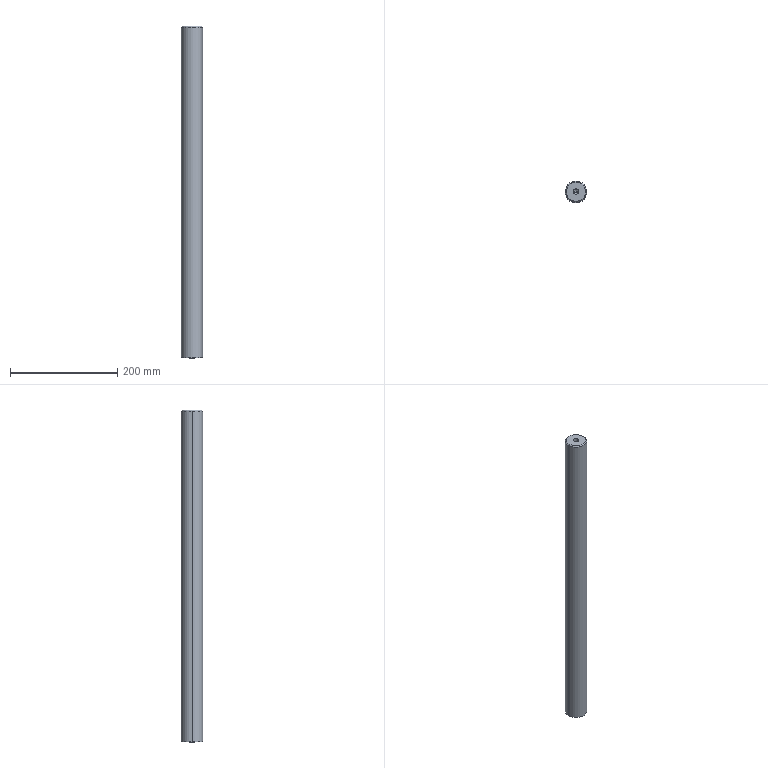Part | STEP file | fBY02F02M-00-02A | 1 solid | 12 faces | box 40 x 40 x 620 mm | volume 776363 mm3 | cone 6 | cylinder 4 | plane 2 | commonest cylinder face diameters 10.2 x2 40 x2
STEP:
#1=CARTESIAN_POINT('',(0.,0.,0.));
#2=DIRECTION('',(0.,0.,1.));
#3=DIRECTION('',(1.,0.,0.));
#4=AXIS2_PLACEMENT_3D('',#1,#2,#3);
#5=CARTESIAN_POINT('',(-20.,0.,648.));
#6=VERTEX_POINT('',#5);
#7=CARTESIAN_POINT('',(20.,0.,648.));
#8=VERTEX_POINT('',#7);
#9=CARTESIAN_POINT('',(0.,0.,648.));
#10=DIRECTION('',(0.,0.,-1.));
#11=DIRECTION('',(-1.,0.,0.));
#12=AXIS2_PLACEMENT_3D('',#9,#10,#11);
#13=CIRCLE('',#12,20.);
#14=CARTESIAN_POINT('',(0.,0.,650.));
#15=DIRECTION('',(0.,0.,-1.));
#16=DIRECTION('',(-1.,0.,0.));
#17=AXIS2_PLACEMENT_3D('',#14,#15,#16);
#18=CYLINDRICAL_SURFACE('',#17,20.);
#19=CARTESIAN_POINT('',(0.,2.));
#20=DIRECTION('',(1.,0.));
#21=VECTOR('',#20,1.);
#22=LINE('',#19,#21);
#23=(GEOMETRIC_REPRESENTATION_CONTEXT(2)PARAMETRIC_REPRESENTATION_CONTEXT()REPRESENTATION_CONTEXT('',''));
#24=DEFINITIONAL_REPRESENTATION('',(#22),#23);
#25=PCURVE('',#18,#24);
#26=CARTESIAN_POINT('',(0.,0.,648.));
#27=DIRECTION('',(0.,0.,-1.));
#28=DIRECTION('',(-1.,0.,0.));
#29=AXIS2_PLACEMENT_3D('',#26,#27,#28);
#30=CONICAL_SURFACE('',#29,20.,0.7854);
#31=CARTESIAN_POINT('',(0.,0.));
#32=DIRECTION('',(1.,0.));
#33=VECTOR('',#32,1.);
#34=LINE('',#31,#33);
#35=(GEOMETRIC_REPRESENTATION_CONTEXT(2)PARAMETRIC_REPRESENTATION_CONTEXT()REPRESENTATION_CONTEXT('',''));
#36=DEFINITIONAL_REPRESENTATION('',(#34),#35);
#37=PCURVE('',#30,#36);
#38=SURFACE_CURVE('',#13,(#25,#37),.PCURVE_S1.);
#39=EDGE_CURVE('',#6,#8,#38,.T.);
#40=ORIENTED_EDGE('',*,*,#39,.T.);
#41=CARTESIAN_POINT('',(20.,0.,30.));
#42=VERTEX_POINT('',#41);
#43=CARTESIAN_POINT('',(20.,0.,650.));
#44=DIRECTION('',(0.,0.,-1.));
#45=VECTOR('',#44,1.);
#46=LINE('',#43,#45);
#47=CARTESIAN_POINT('',(3.142,0.));
#48=DIRECTION('',(0.,1.));
#49=VECTOR('',#48,1.);
#50=LINE('',#47,#49);
#51=(GEOMETRIC_REPRESENTATION_CONTEXT(2)PARAMETRIC_REPRESENTATION_CONTEXT()REPRESENTATION_CONTEXT('',''));
#52=DEFINITIONAL_REPRESENTATION('',(#50),#51);
#53=PCURVE('',#18,#52);
#54=CARTESIAN_POINT('',(0.,0.,650.));
#55=DIRECTION('',(0.,0.,-1.));
#56=DIRECTION('',(-1.,0.,0.));
#57=AXIS2_PLACEMENT_3D('',#54,#55,#56);
#58=CYLINDRICAL_SURFACE('',#57,20.);
#59=CARTESIAN_POINT('',(3.142,0.));
#60=DIRECTION('',(0.,1.));
#61=VECTOR('',#60,1.);
#62=LINE('',#59,#61);
#63=(GEOMETRIC_REPRESENTATION_CONTEXT(2)PARAMETRIC_REPRESENTATION_CONTEXT()REPRESENTATION_CONTEXT('',''));
#64=DEFINITIONAL_REPRESENTATION('',(#62),#63);
#65=PCURVE('',#58,#64);
#66=SURFACE_CURVE('',#46,(#53,#65),.PCURVE_S1.);
#67=EDGE_CURVE('',#8,#42,#66,.T.);
#68=ORIENTED_EDGE('',*,*,#67,.T.);
#69=CARTESIAN_POINT('',(-20.,0.,30.));
#70=VERTEX_POINT('',#69);
#71=CARTESIAN_POINT('',(0.,0.,30.));
#72=DIRECTION('',(0.,0.,1.));
#73=DIRECTION('',(-1.,0.,0.));
#74=AXIS2_PLACEMENT_3D('',#71,#72,#73);
#75=CIRCLE('',#74,20.);
#76=CARTESIAN_POINT('',(6.283,620.));
#77=DIRECTION('',(-1.,0.));
#78=VECTOR('',#77,1.);
#79=LINE('',#76,#78);
#80=(GEOMETRIC_REPRESENTATION_CONTEXT(2)PARAMETRIC_REPRESENTATION_CONTEXT()REPRESENTATION_CONTEXT('',''));
#81=DEFINITIONAL_REPRESENTATION('',(#79),#80);
#82=PCURVE('',#18,#81);
#83=CARTESIAN_POINT('',(0.,0.,30.));
#84=DIRECTION('',(0.,0.,-1.));
#85=DIRECTION('',(-1.,0.,0.));
#86=AXIS2_PLACEMENT_3D('',#83,#84,#85);
#87=PLANE('',#86);
#88=CARTESIAN_POINT('',(20.,0.));
#89=CARTESIAN_POINT('',(20.,-34.641));
#90=CARTESIAN_POINT('',(-10.,-17.321));
#91=CARTESIAN_POINT('',(-40.,0.));
#92=CARTESIAN_POINT('',(-10.,17.321));
#93=CARTESIAN_POINT('',(20.,34.641));
#94=CARTESIAN_POINT('',(20.,0.));
#95=(BOUNDED_CURVE()B_SPLINE_CURVE(2,(#88,#89,#90,#91,#92,#93,#94),.UNSPECIFIED.,.T.,.F.)B_SPLINE_CURVE_WITH_KNOTS((1,2,2,2,2,1),(-2.094,0.,2.094,4.189,6.283,8.378),.UNSPECIFIED.)CURVE()GEOMETRIC_REPRESENTATION_ITEM()RATIONAL_B_SPLINE_CURVE((1.,0.5,1.,0.5,1.,0.5,1.))REPRESENTATION_ITEM(''));
#96=(GEOMETRIC_REPRESENTATION_CONTEXT(2)PARAMETRIC_REPRESENTATION_CONTEXT()REPRESENTATION_CONTEXT('',''));
#97=DEFINITIONAL_REPRESENTATION('',(#95),#96);
#98=PCURVE('',#87,#97);
#99=SURFACE_CURVE('',#75,(#82,#98),.PCURVE_S1.);
#100=EDGE_CURVE('',#42,#70,#99,.T.);
#101=ORIENTED_EDGE('',*,*,#100,.T.);
#102=CARTESIAN_POINT('',(-20.,0.,650.));
#103=DIRECTION('',(0.,0.,-1.));
#104=VECTOR('',#103,1.);
#105=LINE('',#102,#104);
#106=CARTESIAN_POINT('',(0.,0.));
#107=DIRECTION('',(0.,1.));
#108=VECTOR('',#107,1.);
#109=LINE('',#106,#108);
#110=(GEOMETRIC_REPRESENTATION_CONTEXT(2)PARAMETRIC_REPRESENTATION_CONTEXT()REPRESENTATION_CONTEXT('',''));
#111=DEFINITIONAL_REPRESENTATION('',(#109),#110);
#112=PCURVE('',#18,#111);
#113=CARTESIAN_POINT('',(6.283,0.));
#114=DIRECTION('',(0.,1.));
#115=VECTOR('',#114,1.);
#116=LINE('',#113,#115);
#117=(GEOMETRIC_REPRESENTATION_CONTEXT(2)PARAMETRIC_REPRESENTATION_CONTEXT()REPRESENTATION_CONTEXT('',''));
#118=DEFINITIONAL_REPRESENTATION('',(#116),#117);
#119=PCURVE('',#58,#118);
#120=SURFACE_CURVE('',#105,(#112,#119),.PCURVE_S1.);
#121=EDGE_CURVE('',#6,#70,#120,.T.);
#122=ORIENTED_EDGE('',*,*,#121,.F.);
#123=EDGE_LOOP('',(#40,#68,#101,#122));
#124=FACE_BOUND('',#123,.T.);
#125=ADVANCED_FACE('',(#124),#18,.T.);
#126=CARTESIAN_POINT('',(-18.,0.,650.));
#127=VERTEX_POINT('',#126);
#128=CARTESIAN_POINT('',(18.,0.,650.));
#129=VERTEX_POINT('',#128);
#130=CARTESIAN_POINT('',(0.,0.,650.));
#131=DIRECTION('',(0.,0.,-1.));
#132=DIRECTION('',(-1.,0.,0.));
#133=AXIS2_PLACEMENT_3D('',#130,#131,#132);
#134=CIRCLE('',#133,18.);
#135=CARTESIAN_POINT('',(0.,-2.));
#136=DIRECTION('',(1.,0.));
#137=VECTOR('',#136,1.);
#138=LINE('',#135,#137);
#139=(GEOMETRIC_REPRESENTATION_CONTEXT(2)PARAMETRIC_REPRESENTATION_CONTEXT()REPRESENTATION_CONTEXT('',''));
#140=DEFINITIONAL_REPRESENTATION('',(#138),#139);
#141=PCURVE('',#30,#140);
#142=CARTESIAN_POINT('',(0.,0.,650.));
#143=DIRECTION('',(0.,0.,1.));
#144=DIRECTION('',(1.,0.,0.));
#145=AXIS2_PLACEMENT_3D('',#142,#143,#144);
#146=PLANE('',#145);
#147=CARTESIAN_POINT('',(-18.,0.));
#148=CARTESIAN_POINT('',(-18.,31.177));
#149=CARTESIAN_POINT('',(9.,15.588));
#150=CARTESIAN_POINT('',(36.,0.));
#151=CARTESIAN_POINT('',(9.,-15.588));
#152=CARTESIAN_POINT('',(-18.,-31.177));
#153=CARTESIAN_POINT('',(-18.,0.));
#154=(BOUNDED_CURVE()B_SPLINE_CURVE(2,(#147,#148,#149,#150,#151,#152,#153),.UNSPECIFIED.,.T.,.F.)B_SPLINE_CURVE_WITH_KNOTS((1,2,2,2,2,1),(-2.094,0.,2.094,4.189,6.283,8.378),.UNSPECIFIED.)CURVE()GEOMETRIC_REPRESENTATION_ITEM()RATIONAL_B_SPLINE_CURVE((1.,0.5,1.,0.5,1.,0.5,1.))REPRESENTATION_ITEM(''));
#155=(GEOMETRIC_REPRESENTATION_CONTEXT(2)PARAMETRIC_REPRESENTATION_CONTEXT()REPRESENTATION_CONTEXT('',''));
#156=DEFINITIONAL_REPRESENTATION('',(#154),#155);
#157=PCURVE('',#146,#156);
#158=SURFACE_CURVE('',#134,(#141,#157),.PCURVE_S1.);
#159=EDGE_CURVE('',#127,#129,#158,.T.);
#160=ORIENTED_EDGE('',*,*,#159,.T.);
#161=CARTESIAN_POINT('',(20.,0.,648.));
#162=DIRECTION('',(0.7071,0.,-0.7071));
#163=VECTOR('',#162,1.);
#164=LINE('',#161,#163);
#165=CARTESIAN_POINT('',(3.142,0.));
#166=DIRECTION('',(0.,1.));
#167=VECTOR('',#166,1.);
#168=LINE('',#165,#167);
#169=(GEOMETRIC_REPRESENTATION_CONTEXT(2)PARAMETRIC_REPRESENTATION_CONTEXT()REPRESENTATION_CONTEXT('',''));
#170=DEFINITIONAL_REPRESENTATION('',(#168),#169);
#171=PCURVE('',#30,#170);
#172=CARTESIAN_POINT('',(0.,0.,648.));
#173=DIRECTION('',(0.,0.,-1.));
#174=DIRECTION('',(-1.,0.,0.));
#175=AXIS2_PLACEMENT_3D('',#172,#173,#174);
#176=CONICAL_SURFACE('',#175,20.,0.7854);
#177=CARTESIAN_POINT('',(3.142,0.));
#178=DIRECTION('',(0.,1.));
#179=VECTOR('',#178,1.);
#180=LINE('',#177,#179);
#181=(GEOMETRIC_REPRESENTATION_CONTEXT(2)PARAMETRIC_REPRESENTATION_CONTEXT()REPRESENTATION_CONTEXT('',''));
#182=DEFINITIONAL_REPRESENTATION('',(#180),#181);
#183=PCURVE('',#176,#182);
#184=SURFACE_CURVE('',#164,(#171,#183),.PCURVE_S1.);
#185=EDGE_CURVE('',#129,#8,#184,.T.);
#186=ORIENTED_EDGE('',*,*,#185,.T.);
#187=ORIENTED_EDGE('',*,*,#39,.F.);
#188=CARTESIAN_POINT('',(-20.,0.,648.));
#189=DIRECTION('',(-0.7071,0.,-0.7071));
#190=VECTOR('',#189,1.);
#191=LINE('',#188,#190);
#192=CARTESIAN_POINT('',(0.,0.));
#193=DIRECTION('',(0.,1.));
#194=VECTOR('',#193,1.);
#195=LINE('',#192,#194);
#196=(GEOMETRIC_REPRESENTATION_CONTEXT(2)PARAMETRIC_REPRESENTATION_CONTEXT()REPRESENTATION_CONTEXT('',''));
#197=DEFINITIONAL_REPRESENTATION('',(#195),#196);
#198=PCURVE('',#30,#197);
#199=CARTESIAN_POINT('',(6.283,0.));
#200=DIRECTION('',(0.,1.));
#201=VECTOR('',#200,1.);
#202=LINE('',#199,#201);
#203=(GEOMETRIC_REPRESENTATION_CONTEXT(2)PARAMETRIC_REPRESENTATION_CONTEXT()REPRESENTATION_CONTEXT('',''));
#204=DEFINITIONAL_REPRESENTATION('',(#202),#203);
#205=PCURVE('',#176,#204);
#206=SURFACE_CURVE('',#191,(#198,#205),.PCURVE_S1.);
#207=EDGE_CURVE('',#127,#6,#206,.T.);
#208=ORIENTED_EDGE('',*,*,#207,.F.);
#209=EDGE_LOOP('',(#160,#186,#187,#208));
#210=FACE_BOUND('',#209,.T.);
#211=ADVANCED_FACE('',(#210),#30,.T.);
#212=CARTESIAN_POINT('',(0.,3.852,30.));
#213=VERTEX_POINT('',#212);
#214=CARTESIAN_POINT('',(0.,-3.852,30.));
#215=VERTEX_POINT('',#214);
#216=CARTESIAN_POINT('',(0.,0.,30.));
#217=DIRECTION('',(0.,0.,1.));
#218=DIRECTION('',(0.,1.,0.));
#219=AXIS2_PLACEMENT_3D('',#216,#217,#218);
#220=CIRCLE('',#219,3.852);
#221=CARTESIAN_POINT('',(0.,0.,30.));
#222=DIRECTION('',(0.,0.,-1.));
#223=DIRECTION('',(0.,1.,0.));
#224=AXIS2_PLACEMENT_3D('',#221,#222,#223);
#225=CONICAL_SURFACE('',#224,3.852,1.03);
#226=CARTESIAN_POINT('',(6.283,0.));
#227=DIRECTION('',(-1.,0.));
#228=VECTOR('',#227,1.);
#229=LINE('',#226,#228);
#230=(GEOMETRIC_REPRESENTATION_CONTEXT(2)PARAMETRIC_REPRESENTATION_CONTEXT()REPRESENTATION_CONTEXT('',''));
#231=DEFINITIONAL_REPRESENTATION('',(#229),#230);
#232=PCURVE('',#225,#231);
#233=CARTESIAN_POINT('',(0.,3.852));
#234=CARTESIAN_POINT('',(6.671,3.852));
#235=CARTESIAN_POINT('',(3.336,-1.926));
#236=CARTESIAN_POINT('',(0.,-7.704));
#237=CARTESIAN_POINT('',(-3.336,-1.926));
#238=CARTESIAN_POINT('',(-6.671,3.852));
#239=CARTESIAN_POINT('',(0.,3.852));
#240=(BOUNDED_CURVE()B_SPLINE_CURVE(2,(#233,#234,#235,#236,#237,#238,#239),.UNSPECIFIED.,.T.,.F.)B_SPLINE_CURVE_WITH_KNOTS((1,2,2,2,2,1),(-2.094,0.,2.094,4.189,6.283,8.378),.UNSPECIFIED.)CURVE()GEOMETRIC_REPRESENTATION_ITEM()RATIONAL_B_SPLINE_CURVE((1.,0.5,1.,0.5,1.,0.5,1.))REPRESENTATION_ITEM(''));
#241=(GEOMETRIC_REPRESENTATION_CONTEXT(2)PARAMETRIC_REPRESENTATION_CONTEXT()REPRESENTATION_CONTEXT('',''));
#242=DEFINITIONAL_REPRESENTATION('',(#240),#241);
#243=PCURVE('',#87,#242);
#244=SURFACE_CURVE('',#220,(#232,#243),.PCURVE_S1.);
#245=EDGE_CURVE('',#213,#215,#244,.T.);
#246=ORIENTED_EDGE('',*,*,#245,.T.);
#247=CARTESIAN_POINT('',(0.,0.,32.314));
#248=VERTEX_POINT('',#247);
#249=CARTESIAN_POINT('',(0.,-3.852,30.));
#250=DIRECTION('',(0.,-0.8572,-0.515));
#251=VECTOR('',#250,1.);
#252=LINE('',#249,#251);
#253=CARTESIAN_POINT('',(3.142,0.));
#254=DIRECTION('',(0.,1.));
#255=VECTOR('',#254,1.);
#256=LINE('',#253,#255);
#257=(GEOMETRIC_REPRESENTATION_CONTEXT(2)PARAMETRIC_REPRESENTATION_CONTEXT()REPRESENTATION_CONTEXT('',''));
#258=DEFINITIONAL_REPRESENTATION('',(#256),#257);
#259=PCURVE('',#225,#258);
#260=CARTESIAN_POINT('',(0.,0.,30.));
#261=DIRECTION('',(0.,0.,-1.));
#262=DIRECTION('',(0.,1.,0.));
#263=AXIS2_PLACEMENT_3D('',#260,#261,#262);
#264=CONICAL_SURFACE('',#263,3.852,1.03);
#265=CARTESIAN_POINT('',(3.142,0.));
#266=DIRECTION('',(0.,1.));
#267=VECTOR('',#266,1.);
#268=LINE('',#265,#267);
#269=(GEOMETRIC_REPRESENTATION_CONTEXT(2)PARAMETRIC_REPRESENTATION_CONTEXT()REPRESENTATION_CONTEXT('',''));
#270=DEFINITIONAL_REPRESENTATION('',(#268),#269);
#271=PCURVE('',#264,#270);
#272=SURFACE_CURVE('',#252,(#259,#271),.PCURVE_S1.);
#273=EDGE_CURVE('',#248,#215,#272,.T.);
#274=ORIENTED_EDGE('',*,*,#273,.F.);
#275=CARTESIAN_POINT('',(0.,3.852,30.));
#276=DIRECTION('',(0.,0.8572,-0.515));
#277=VECTOR('',#276,1.);
#278=LINE('',#275,#277);
#279=CARTESIAN_POINT('',(6.283,0.));
#280=DIRECTION('',(0.,1.));
#281=VECTOR('',#280,1.);
#282=LINE('',#279,#281);
#283=(GEOMETRIC_REPRESENTATION_CONTEXT(2)PARAMETRIC_REPRESENTATION_CONTEXT()REPRESENTATION_CONTEXT('',''));
#284=DEFINITIONAL_REPRESENTATION('',(#282),#283);
#285=PCURVE('',#225,#284);
#286=CARTESIAN_POINT('',(0.,0.));
#287=DIRECTION('',(0.,1.));
#288=VECTOR('',#287,1.);
#289=LINE('',#286,#288);
#290=(GEOMETRIC_REPRESENTATION_CONTEXT(2)PARAMETRIC_REPRESENTATION_CONTEXT()REPRESENTATION_CONTEXT('',''));
#291=DEFINITIONAL_REPRESENTATION('',(#289),#290);
#292=PCURVE('',#264,#291);
#293=SURFACE_CURVE('',#278,(#285,#292),.PCURVE_S1.);
#294=EDGE_CURVE('',#248,#213,#293,.T.);
#295=ORIENTED_EDGE('',*,*,#294,.T.);
#296=EDGE_LOOP('',(#246,#274,#295));
#297=FACE_BOUND('',#296,.F.);
#298=ADVANCED_FACE('',(#297),#225,.F.);
#299=CARTESIAN_POINT('',(5.1,0.,620.75));
#300=VERTEX_POINT('',#299);
#301=CARTESIAN_POINT('',(5.1,0.,650.));
#302=VERTEX_POINT('',#301);
#303=CARTESIAN_POINT('',(5.1,0.,650.));
#304=DIRECTION('',(0.,0.,1.));
#305=VECTOR('',#304,1.);
#306=LINE('',#303,#305);
#307=CARTESIAN_POINT('',(0.,0.,650.));
#308=DIRECTION('',(0.,0.,1.));
#309=DIRECTION('',(1.,0.,0.));
#310=AXIS2_PLACEMENT_3D('',#307,#308,#309);
#311=CYLINDRICAL_SURFACE('',#310,5.1);
#312=CARTESIAN_POINT('',(6.283,0.));
#313=DIRECTION('',(0.,1.));
#314=VECTOR('',#313,1.);
#315=LINE('',#312,#314);
#316=(GEOMETRIC_REPRESENTATION_CONTEXT(2)PARAMETRIC_REPRESENTATION_CONTEXT()REPRESENTATION_CONTEXT('',''));
#317=DEFINITIONAL_REPRESENTATION('',(#315),#316);
#318=PCURVE('',#311,#317);
#319=CARTESIAN_POINT('',(0.,0.,650.));
#320=DIRECTION('',(0.,0.,1.));
#321=DIRECTION('',(1.,0.,0.));
#322=AXIS2_PLACEMENT_3D('',#319,#320,#321);
#323=CYLINDRICAL_SURFACE('',#322,5.1);
#324=CARTESIAN_POINT('',(0.,0.));
#325=DIRECTION('',(0.,1.));
#326=VECTOR('',#325,1.);
#327=LINE('',#324,#326);
#328=(GEOMETRIC_REPRESENTATION_CONTEXT(2)PARAMETRIC_REPRESENTATION_CONTEXT()REPRESENTATION_CONTEXT('',''));
#329=DEFINITIONAL_REPRESENTATION('',(#327),#328);
#330=PCURVE('',#323,#329);
#331=SURFACE_CURVE('',#306,(#318,#330),.PCURVE_S1.);
#332=EDGE_CURVE('',#300,#302,#331,.T.);
#333=ORIENTED_EDGE('',*,*,#332,.T.);
#334=CARTESIAN_POINT('',(-5.1,0.,650.));
#335=VERTEX_POINT('',#334);
#336=CARTESIAN_POINT('',(0.,0.,650.));
#337=DIRECTION('',(0.,0.,-1.));
#338=DIRECTION('',(1.,0.,0.));
#339=AXIS2_PLACEMENT_3D('',#336,#337,#338);
#340=CIRCLE('',#339,5.1);
#341=CARTESIAN_POINT('',(6.283,0.));
#342=DIRECTION('',(-1.,0.));
#343=VECTOR('',#342,1.);
#344=LINE('',#341,#343);
#345=(GEOMETRIC_REPRESENTATION_CONTEXT(2)PARAMETRIC_REPRESENTATION_CONTEXT()REPRESENTATION_CONTEXT('',''));
#346=DEFINITIONAL_REPRESENTATION('',(#344),#345);
#347=PCURVE('',#311,#346);
#348=CARTESIAN_POINT('',(5.1,0.));
#349=CARTESIAN_POINT('',(5.1,-8.833));
#350=CARTESIAN_POINT('',(-2.55,-4.417));
#351=CARTESIAN_POINT('',(-10.2,0.));
#352=CARTESIAN_POINT('',(-2.55,4.417));
#353=CARTESIAN_POINT('',(5.1,8.833));
#354=CARTESIAN_POINT('',(5.1,0.));
#355=(BOUNDED_CURVE()B_SPLINE_CURVE(2,(#348,#349,#350,#351,#352,#353,#354),.UNSPECIFIED.,.T.,.F.)B_SPLINE_CURVE_WITH_KNOTS((1,2,2,2,2,1),(-2.094,0.,2.094,4.189,6.283,8.378),.UNSPECIFIED.)CURVE()GEOMETRIC_REPRESENTATION_ITEM()RATIONAL_B_SPLINE_CURVE((1.,0.5,1.,0.5,1.,0.5,1.))REPRESENTATION_ITEM(''));
#356=(GEOMETRIC_REPRESENTATION_CONTEXT(2)PARAMETRIC_REPRESENTATION_CONTEXT()REPRESENTATION_CONTEXT('',''));
#357=DEFINITIONAL_REPRESENTATION('',(#355),#356);
#358=PCURVE('',#146,#357);
#359=SURFACE_CURVE('',#340,(#347,#358),.PCURVE_S1.);
#360=EDGE_CURVE('',#302,#335,#359,.T.);
#361=ORIENTED_EDGE('',*,*,#360,.T.);
#362=CARTESIAN_POINT('',(-5.1,0.,620.75));
#363=VERTEX_POINT('',#362);
#364=CARTESIAN_POINT('',(-5.1,0.,650.));
#365=DIRECTION('',(0.,0.,1.));
#366=VECTOR('',#365,1.);
#367=LINE('',#364,#366);
#368=CARTESIAN_POINT('',(3.142,0.));
#369=DIRECTION('',(0.,1.));
#370=VECTOR('',#369,1.);
#371=LINE('',#368,#370);
#372=(GEOMETRIC_REPRESENTATION_CONTEXT(2)PARAMETRIC_REPRESENTATION_CONTEXT()REPRESENTATION_CONTEXT('',''));
#373=DEFINITIONAL_REPRESENTATION('',(#371),#372);
#374=PCURVE('',#311,#373);
#375=CARTESIAN_POINT('',(3.142,0.));
#376=DIRECTION('',(0.,1.));
#377=VECTOR('',#376,1.);
#378=LINE('',#375,#377);
#379=(GEOMETRIC_REPRESENTATION_CONTEXT(2)PARAMETRIC_REPRESENTATION_CONTEXT()REPRESENTATION_CONTEXT('',''));
#380=DEFINITIONAL_REPRESENTATION('',(#378),#379);
#381=PCURVE('',#323,#380);
#382=SURFACE_CURVE('',#367,(#374,#381),.PCURVE_S1.);
#383=EDGE_CURVE('',#363,#335,#382,.T.);
#384=ORIENTED_EDGE('',*,*,#383,.F.);
#385=CARTESIAN_POINT('',(0.,0.,620.75));
#386=DIRECTION('',(0.,0.,1.));
#387=DIRECTION('',(1.,0.,0.));
#388=AXIS2_PLACEMENT_3D('',#385,#386,#387);
#389=CIRCLE('',#388,5.1);
#390=CARTESIAN_POINT('',(0.,-29.25));
#391=DIRECTION('',(1.,0.));
#392=VECTOR('',#391,1.);
#393=LINE('',#390,#392);
#394=(GEOMETRIC_REPRESENTATION_CONTEXT(2)PARAMETRIC_REPRESENTATION_CONTEXT()REPRESENTATION_CONTEXT('',''));
#395=DEFINITIONAL_REPRESENTATION('',(#393),#394);
#396=PCURVE('',#311,#395);
#397=CARTESIAN_POINT('',(0.,0.,620.75));
#398=DIRECTION('',(0.,0.,1.));
#399=DIRECTION('',(1.,0.,0.));
#400=AXIS2_PLACEMENT_3D('',#397,#398,#399);
#401=CONICAL_SURFACE('',#400,5.1,1.03);
#402=CARTESIAN_POINT('',(0.,0.));
#403=DIRECTION('',(1.,0.));
#404=VECTOR('',#403,1.);
#405=LINE('',#402,#404);
#406=(GEOMETRIC_REPRESENTATION_CONTEXT(2)PARAMETRIC_REPRESENTATION_CONTEXT()REPRESENTATION_CONTEXT('',''));
#407=DEFINITIONAL_REPRESENTATION('',(#405),#406);
#408=PCURVE('',#401,#407);
#409=SURFACE_CURVE('',#389,(#396,#408),.PCURVE_S1.);
#410=EDGE_CURVE('',#363,#300,#409,.T.);
#411=ORIENTED_EDGE('',*,*,#410,.T.);
#412=EDGE_LOOP('',(#333,#361,#384,#411));
#413=FACE_BOUND('',#412,.F.);
#414=ADVANCED_FACE('',(#413),#311,.F.);
#415=ORIENTED_EDGE('',*,*,#410,.F.);
#416=CARTESIAN_POINT('',(0.,0.,617.686));
#417=VERTEX_POINT('',#416);
#418=CARTESIAN_POINT('',(-5.1,0.,620.75));
#419=DIRECTION('',(-0.8572,0.,0.515));
#420=VECTOR('',#419,1.);
#421=LINE('',#418,#420);
#422=CARTESIAN_POINT('',(3.142,0.));
#423=DIRECTION('',(0.,1.));
#424=VECTOR('',#423,1.);
#425=LINE('',#422,#424);
#426=(GEOMETRIC_REPRESENTATION_CONTEXT(2)PARAMETRIC_REPRESENTATION_CONTEXT()REPRESENTATION_CONTEXT('',''));
#427=DEFINITIONAL_REPRESENTATION('',(#425),#426);
#428=PCURVE('',#401,#427);
#429=CARTESIAN_POINT('',(0.,0.,620.75));
#430=DIRECTION('',(0.,0.,1.));
#431=DIRECTION('',(1.,0.,0.));
#432=AXIS2_PLACEMENT_3D('',#429,#430,#431);
#433=CONICAL_SURFACE('',#432,5.1,1.03);
#434=CARTESIAN_POINT('',(3.142,0.));
#435=DIRECTION('',(0.,1.));
#436=VECTOR('',#435,1.);
#437=LINE('',#434,#436);
#438=(GEOMETRIC_REPRESENTATION_CONTEXT(2)PARAMETRIC_REPRESENTATION_CONTEXT()REPRESENTATION_CONTEXT('',''));
#439=DEFINITIONAL_REPRESENTATION('',(#437),#438);
#440=PCURVE('',#433,#439);
#441=SURFACE_CURVE('',#421,(#428,#440),.PCURVE_S1.);
#442=EDGE_CURVE('',#417,#363,#441,.T.);
#443=ORIENTED_EDGE('',*,*,#442,.F.);
#444=CARTESIAN_POINT('',(5.1,0.,620.75));
#445=DIRECTION('',(0.8572,0.,0.515));
#446=VECTOR('',#445,1.);
#447=LINE('',#444,#446);
#448=CARTESIAN_POINT('',(6.283,0.));
#449=DIRECTION('',(0.,1.));
#450=VECTOR('',#449,1.);
#451=LINE('',#448,#450);
#452=(GEOMETRIC_REPRESENTATION_CONTEXT(2)PARAMETRIC_REPRESENTATION_CONTEXT()REPRESENTATION_CONTEXT('',''));
#453=DEFINITIONAL_REPRESENTATION('',(#451),#452);
#454=PCURVE('',#401,#453);
#455=CARTESIAN_POINT('',(0.,0.));
#456=DIRECTION('',(0.,1.));
#457=VECTOR('',#456,1.);
#458=LINE('',#455,#457);
#459=(GEOMETRIC_REPRESENTATION_CONTEXT(2)PARAMETRIC_REPRESENTATION_CONTEXT()REPRESENTATION_CONTEXT('',''));
#460=DEFINITIONAL_REPRESENTATION('',(#458),#459);
#461=PCURVE('',#433,#460);
#462=SURFACE_CURVE('',#447,(#454,#461),.PCURVE_S1.);
#463=EDGE_CURVE('',#417,#300,#462,.T.);
#464=ORIENTED_EDGE('',*,*,#463,.T.);
#465=EDGE_LOOP('',(#415,#443,#464));
#466=FACE_BOUND('',#465,.F.);
#467=ADVANCED_FACE('',(#466),#401,.F.);
#468=ORIENTED_EDGE('',*,*,#67,.F.);
#469=CARTESIAN_POINT('',(0.,0.,648.));
#470=DIRECTION('',(0.,0.,-1.));
#471=DIRECTION('',(-1.,0.,0.));
#472=AXIS2_PLACEMENT_3D('',#469,#470,#471);
#473=CIRCLE('',#472,20.);
#474=CARTESIAN_POINT('',(0.,2.));
#475=DIRECTION('',(1.,0.));
#476=VECTOR('',#475,1.);
#477=LINE('',#474,#476);
#478=(GEOMETRIC_REPRESENTATION_CONTEXT(2)PARAMETRIC_REPRESENTATION_CONTEXT()REPRESENTATION_CONTEXT('',''));
#479=DEFINITIONAL_REPRESENTATION('',(#477),#478);
#480=PCURVE('',#58,#479);
#481=CARTESIAN_POINT('',(0.,0.));
#482=DIRECTION('',(1.,0.));
#483=VECTOR('',#482,1.);
#484=LINE('',#481,#483);
#485=(GEOMETRIC_REPRESENTATION_CONTEXT(2)PARAMETRIC_REPRESENTATION_CONTEXT()REPRESENTATION_CONTEXT('',''));
#486=DEFINITIONAL_REPRESENTATION('',(#484),#485);
#487=PCURVE('',#176,#486);
#488=SURFACE_CURVE('',#473,(#480,#487),.PCURVE_S1.);
#489=EDGE_CURVE('',#8,#6,#488,.T.);
#490=ORIENTED_EDGE('',*,*,#489,.T.);
#491=ORIENTED_EDGE('',*,*,#121,.T.);
#492=CARTESIAN_POINT('',(0.,0.,30.));
#493=DIRECTION('',(0.,0.,1.));
#494=DIRECTION('',(-1.,0.,0.));
#495=AXIS2_PLACEMENT_3D('',#492,#493,#494);
#496=CIRCLE('',#495,20.);
#497=CARTESIAN_POINT('',(6.283,620.));
#498=DIRECTION('',(-1.,0.));
#499=VECTOR('',#498,1.);
#500=LINE('',#497,#499);
#501=(GEOMETRIC_REPRESENTATION_CONTEXT(2)PARAMETRIC_REPRESENTATION_CONTEXT()REPRESENTATION_CONTEXT('',''));
#502=DEFINITIONAL_REPRESENTATION('',(#500),#501);
#503=PCURVE('',#58,#502);
#504=CARTESIAN_POINT('',(20.,0.));
#505=CARTESIAN_POINT('',(20.,-34.641));
#506=CARTESIAN_POINT('',(-10.,-17.321));
#507=CARTESIAN_POINT('',(-40.,0.));
#508=CARTESIAN_POINT('',(-10.,17.321));
#509=CARTESIAN_POINT('',(20.,34.641));
#510=CARTESIAN_POINT('',(20.,0.));
#511=(BOUNDED_CURVE()B_SPLINE_CURVE(2,(#504,#505,#506,#507,#508,#509,#510),.UNSPECIFIED.,.T.,.F.)B_SPLINE_CURVE_WITH_KNOTS((1,2,2,2,2,1),(-2.094,0.,2.094,4.189,6.283,8.378),.UNSPECIFIED.)CURVE()GEOMETRIC_REPRESENTATION_ITEM()RATIONAL_B_SPLINE_CURVE((1.,0.5,1.,0.5,1.,0.5,1.))REPRESENTATION_ITEM(''));
#512=(GEOMETRIC_REPRESENTATION_CONTEXT(2)PARAMETRIC_REPRESENTATION_CONTEXT()REPRESENTATION_CONTEXT('',''));
#513=DEFINITIONAL_REPRESENTATION('',(#511),#512);
#514=PCURVE('',#87,#513);
#515=SURFACE_CURVE('',#496,(#503,#514),.PCURVE_S1.);
#516=EDGE_CURVE('',#70,#42,#515,.T.);
#517=ORIENTED_EDGE('',*,*,#516,.T.);
#518=EDGE_LOOP('',(#468,#490,#491,#517));
#519=FACE_BOUND('',#518,.T.);
#520=ADVANCED_FACE('',(#519),#58,.T.);
#521=ORIENTED_EDGE('',*,*,#516,.F.);
#522=ORIENTED_EDGE('',*,*,#100,.F.);
#523=EDGE_LOOP('',(#521,#522));
#524=FACE_BOUND('',#523,.T.);
#525=ORIENTED_EDGE('',*,*,#245,.T.);
#526=CARTESIAN_POINT('',(0.,0.,30.));
#527=DIRECTION('',(0.,0.,1.));
#528=DIRECTION('',(0.,1.,0.));
#529=AXIS2_PLACEMENT_3D('',#526,#527,#528);
#530=CIRCLE('',#529,3.852);
#531=CARTESIAN_POINT('',(0.,3.852));
#532=CARTESIAN_POINT('',(6.671,3.852));
#533=CARTESIAN_POINT('',(3.336,-1.926));
#534=CARTESIAN_POINT('',(0.,-7.704));
#535=CARTESIAN_POINT('',(-3.336,-1.926));
#536=CARTESIAN_POINT('',(-6.671,3.852));
#537=CARTESIAN_POINT('',(0.,3.852));
#538=(BOUNDED_CURVE()B_SPLINE_CURVE(2,(#531,#532,#533,#534,#535,#536,#537),.UNSPECIFIED.,.T.,.F.)B_SPLINE_CURVE_WITH_KNOTS((1,2,2,2,2,1),(-2.094,0.,2.094,4.189,6.283,8.378),.UNSPECIFIED.)CURVE()GEOMETRIC_REPRESENTATION_ITEM()RATIONAL_B_SPLINE_CURVE((1.,0.5,1.,0.5,1.,0.5,1.))REPRESENTATION_ITEM(''));
#539=(GEOMETRIC_REPRESENTATION_CONTEXT(2)PARAMETRIC_REPRESENTATION_CONTEXT()REPRESENTATION_CONTEXT('',''));
#540=DEFINITIONAL_REPRESENTATION('',(#538),#539);
#541=PCURVE('',#87,#540);
#542=CARTESIAN_POINT('',(6.283,0.));
#543=DIRECTION('',(-1.,0.));
#544=VECTOR('',#543,1.);
#545=LINE('',#542,#544);
#546=(GEOMETRIC_REPRESENTATION_CONTEXT(2)PARAMETRIC_REPRESENTATION_CONTEXT()REPRESENTATION_CONTEXT('',''));
#547=DEFINITIONAL_REPRESENTATION('',(#545),#546);
#548=PCURVE('',#264,#547);
#549=SURFACE_CURVE('',#530,(#541,#548),.PCURVE_S1.);
#550=EDGE_CURVE('',#215,#213,#549,.T.);
#551=ORIENTED_EDGE('',*,*,#550,.T.);
#552=EDGE_LOOP('',(#525,#551));
#553=FACE_BOUND('',#552,.T.);
#554=ADVANCED_FACE('',(#524,#553),#87,.T.);
#555=ORIENTED_EDGE('',*,*,#185,.F.);
#556=CARTESIAN_POINT('',(0.,0.,650.));
#557=DIRECTION('',(0.,0.,-1.));
#558=DIRECTION('',(-1.,0.,0.));
#559=AXIS2_PLACEMENT_3D('',#556,#557,#558);
#560=CIRCLE('',#559,18.);
#561=CARTESIAN_POINT('',(0.,-2.));
#562=DIRECTION('',(1.,0.));
#563=VECTOR('',#562,1.);
#564=LINE('',#561,#563);
#565=(GEOMETRIC_REPRESENTATION_CONTEXT(2)PARAMETRIC_REPRESENTATION_CONTEXT()REPRESENTATION_CONTEXT('',''));
#566=DEFINITIONAL_REPRESENTATION('',(#564),#565);
#567=PCURVE('',#176,#566);
#568=CARTESIAN_POINT('',(-18.,0.));
#569=CARTESIAN_POINT('',(-18.,31.177));
#570=CARTESIAN_POINT('',(9.,15.588));
#571=CARTESIAN_POINT('',(36.,0.));
#572=CARTESIAN_POINT('',(9.,-15.588));
#573=CARTESIAN_POINT('',(-18.,-31.177));
#574=CARTESIAN_POINT('',(-18.,0.));
#575=(BOUNDED_CURVE()B_SPLINE_CURVE(2,(#568,#569,#570,#571,#572,#573,#574),.UNSPECIFIED.,.T.,.F.)B_SPLINE_CURVE_WITH_KNOTS((1,2,2,2,2,1),(-2.094,0.,2.094,4.189,6.283,8.378),.UNSPECIFIED.)CURVE()GEOMETRIC_REPRESENTATION_ITEM()RATIONAL_B_SPLINE_CURVE((1.,0.5,1.,0.5,1.,0.5,1.))REPRESENTATION_ITEM(''));
#576=(GEOMETRIC_REPRESENTATION_CONTEXT(2)PARAMETRIC_REPRESENTATION_CONTEXT()REPRESENTATION_CONTEXT('',''));
#577=DEFINITIONAL_REPRESENTATION('',(#575),#576);
#578=PCURVE('',#146,#577);
#579=SURFACE_CURVE('',#560,(#567,#578),.PCURVE_S1.);
#580=EDGE_CURVE('',#129,#127,#579,.T.);
#581=ORIENTED_EDGE('',*,*,#580,.T.);
#582=ORIENTED_EDGE('',*,*,#207,.T.);
#583=ORIENTED_EDGE('',*,*,#489,.F.);
#584=EDGE_LOOP('',(#555,#581,#582,#583));
#585=FACE_BOUND('',#584,.T.);
#586=ADVANCED_FACE('',(#585),#176,.T.);
#587=ORIENTED_EDGE('',*,*,#550,.T.);
#588=ORIENTED_EDGE('',*,*,#294,.F.);
#589=ORIENTED_EDGE('',*,*,#273,.T.);
#590=EDGE_LOOP('',(#587,#588,#589));
#591=FACE_BOUND('',#590,.F.);
#592=ADVANCED_FACE('',(#591),#264,.F.);
#593=ORIENTED_EDGE('',*,*,#360,.T.);
#594=CARTESIAN_POINT('',(0.,0.,650.));
#595=DIRECTION('',(0.,0.,-1.));
#596=DIRECTION('',(1.,0.,0.));
#597=AXIS2_PLACEMENT_3D('',#594,#595,#596);
#598=CIRCLE('',#597,5.1);
#599=CARTESIAN_POINT('',(5.1,0.));
#600=CARTESIAN_POINT('',(5.1,-8.833));
#601=CARTESIAN_POINT('',(-2.55,-4.417));
#602=CARTESIAN_POINT('',(-10.2,0.));
#603=CARTESIAN_POINT('',(-2.55,4.417));
#604=CARTESIAN_POINT('',(5.1,8.833));
#605=CARTESIAN_POINT('',(5.1,0.));
#606=(BOUNDED_CURVE()B_SPLINE_CURVE(2,(#599,#600,#601,#602,#603,#604,#605),.UNSPECIFIED.,.T.,.F.)B_SPLINE_CURVE_WITH_KNOTS((1,2,2,2,2,1),(-2.094,0.,2.094,4.189,6.283,8.378),.UNSPECIFIED.)CURVE()GEOMETRIC_REPRESENTATION_ITEM()RATIONAL_B_SPLINE_CURVE((1.,0.5,1.,0.5,1.,0.5,1.))REPRESENTATION_ITEM(''));
#607=(GEOMETRIC_REPRESENTATION_CONTEXT(2)PARAMETRIC_REPRESENTATION_CONTEXT()REPRESENTATION_CONTEXT('',''));
#608=DEFINITIONAL_REPRESENTATION('',(#606),#607);
#609=PCURVE('',#146,#608);
#610=CARTESIAN_POINT('',(6.283,0.));
#611=DIRECTION('',(-1.,0.));
#612=VECTOR('',#611,1.);
#613=LINE('',#610,#612);
#614=(GEOMETRIC_REPRESENTATION_CONTEXT(2)PARAMETRIC_REPRESENTATION_CONTEXT()REPRESENTATION_CONTEXT('',''));
#615=DEFINITIONAL_REPRESENTATION('',(#613),#614);
#616=PCURVE('',#323,#615);
#617=SURFACE_CURVE('',#598,(#609,#616),.PCURVE_S1.);
#618=EDGE_CURVE('',#335,#302,#617,.T.);
#619=ORIENTED_EDGE('',*,*,#618,.T.);
#620=EDGE_LOOP('',(#593,#619));
#621=FACE_BOUND('',#620,.T.);
#622=ORIENTED_EDGE('',*,*,#159,.F.);
#623=ORIENTED_EDGE('',*,*,#580,.F.);
#624=EDGE_LOOP('',(#622,#623));
#625=FACE_BOUND('',#624,.T.);
#626=ADVANCED_FACE('',(#621,#625),#146,.T.);
#627=ORIENTED_EDGE('',*,*,#618,.T.);
#628=ORIENTED_EDGE('',*,*,#332,.F.);
#629=CARTESIAN_POINT('',(0.,0.,620.75));
#630=DIRECTION('',(0.,0.,1.));
#631=DIRECTION('',(1.,0.,0.));
#632=AXIS2_PLACEMENT_3D('',#629,#630,#631);
#633=CIRCLE('',#632,5.1);
#634=CARTESIAN_POINT('',(0.,-29.25));
#635=DIRECTION('',(1.,0.));
#636=VECTOR('',#635,1.);
#637=LINE('',#634,#636);
#638=(GEOMETRIC_REPRESENTATION_CONTEXT(2)PARAMETRIC_REPRESENTATION_CONTEXT()REPRESENTATION_CONTEXT('',''));
#639=DEFINITIONAL_REPRESENTATION('',(#637),#638);
#640=PCURVE('',#323,#639);
#641=CARTESIAN_POINT('',(0.,0.));
#642=DIRECTION('',(1.,0.));
#643=VECTOR('',#642,1.);
#644=LINE('',#641,#643);
#645=(GEOMETRIC_REPRESENTATION_CONTEXT(2)PARAMETRIC_REPRESENTATION_CONTEXT()REPRESENTATION_CONTEXT('',''));
#646=DEFINITIONAL_REPRESENTATION('',(#644),#645);
#647=PCURVE('',#433,#646);
#648=SURFACE_CURVE('',#633,(#640,#647),.PCURVE_S1.);
#649=EDGE_CURVE('',#300,#363,#648,.T.);
#650=ORIENTED_EDGE('',*,*,#649,.T.);
#651=ORIENTED_EDGE('',*,*,#383,.T.);
#652=EDGE_LOOP('',(#627,#628,#650,#651));
#653=FACE_BOUND('',#652,.F.);
#654=ADVANCED_FACE('',(#653),#323,.F.);
#655=ORIENTED_EDGE('',*,*,#649,.F.);
#656=ORIENTED_EDGE('',*,*,#463,.F.);
#657=ORIENTED_EDGE('',*,*,#442,.T.);
#658=EDGE_LOOP('',(#655,#656,#657));
#659=FACE_BOUND('',#658,.F.);
#660=ADVANCED_FACE('',(#659),#433,.F.);
#661=CLOSED_SHELL('',(#125,#211,#298,#414,#467,#520,#554,#586,#592,#626,#654,#660));
#662=MANIFOLD_SOLID_BREP('',#661);
#663=(LENGTH_UNIT()NAMED_UNIT(*)SI_UNIT(.MILLI.,.METRE.));
#664=UNCERTAINTY_MEASURE_WITH_UNIT(LENGTH_MEASURE(0.0000001),#663,'','');
#665=(NAMED_UNIT(*)PLANE_ANGLE_UNIT()SI_UNIT($,.RADIAN.));
#666=(NAMED_UNIT(*)SI_UNIT($,.STERADIAN.)SOLID_ANGLE_UNIT());
#667=(GEOMETRIC_REPRESENTATION_CONTEXT(3)GLOBAL_UNCERTAINTY_ASSIGNED_CONTEXT((#664))GLOBAL_UNIT_ASSIGNED_CONTEXT((#663,#665,#666))REPRESENTATION_CONTEXT('',''));
#668=ADVANCED_BREP_SHAPE_REPRESENTATION('',(#4,#662),#667);